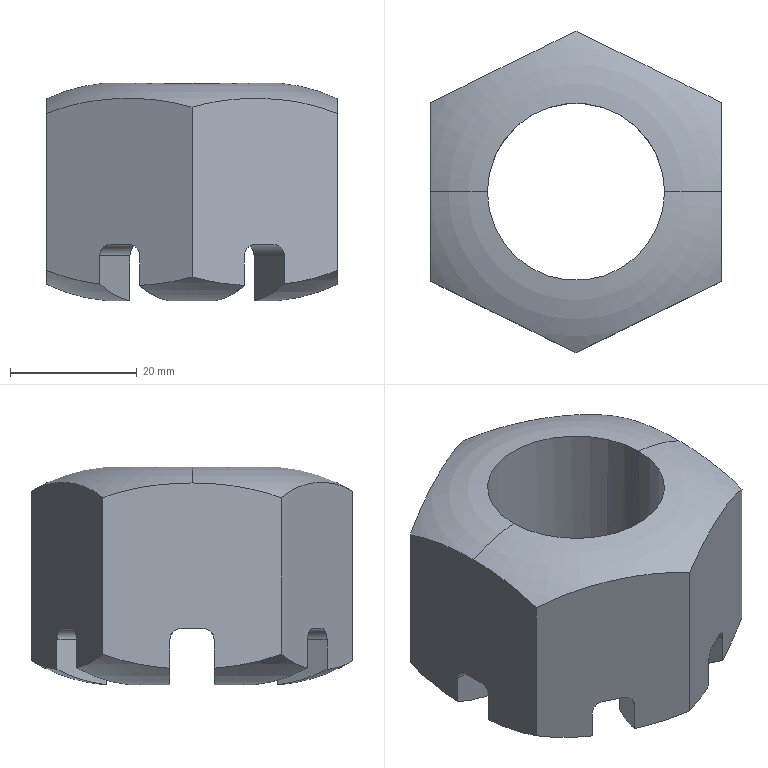Part | SolidWorks | features CirPattern 1, Extrusion 1, Fillet 1, HoleWzd 1, ICE 1, RefAxis 1, RevCut 1 | 1 solid | 46 faces | box 46 x 50.85 x 34.366 mm | volume 35234 mm3 | plane 24 | cylinder 14 | torus 8 | commonest cylinder face diameters 3.6 x12 28 x2